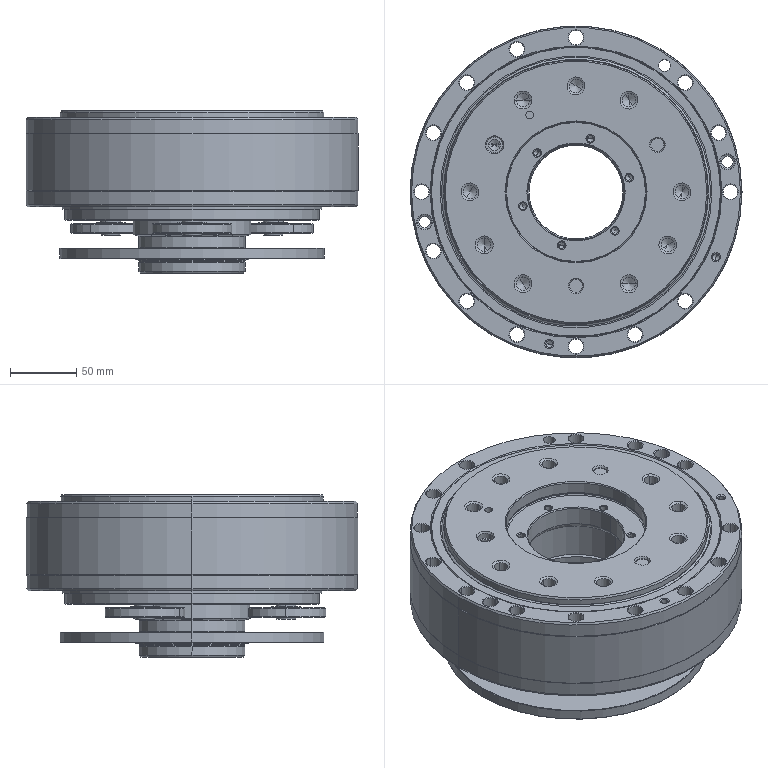Part | SolidWorks | features BaseBody 1 | 1 solid | 587 faces | box 250.5 x 250.5 x 122.6 mm | volume 3466893 mm3 | cone 240 | cylinder 225 | plane 106 | torus 16 | commonest cylinder face diameters 11 x32 10.2 x18 5 x16 15 x12 16 x12 17 x12